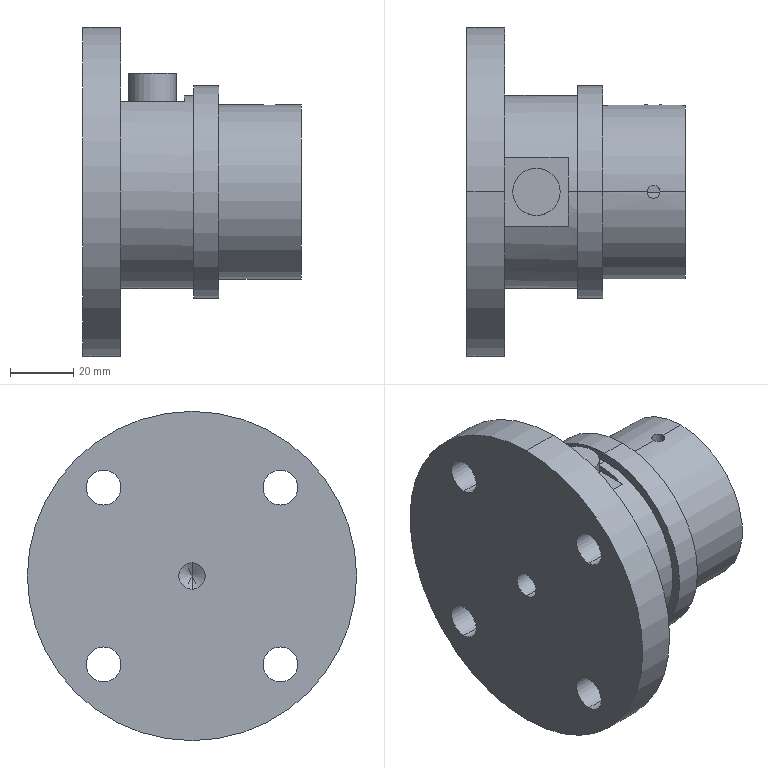Part | STEP file | CLT-50(20220226) | 1 solid | 39 faces | box 69 x 104 x 104 mm | volume 248034 mm3 | cylinder 28 | plane 9 | cone 2 | commonest cylinder face diameters 11 x8 4.134 x4 8.376 x4 15 x2 20 x2 55 x2